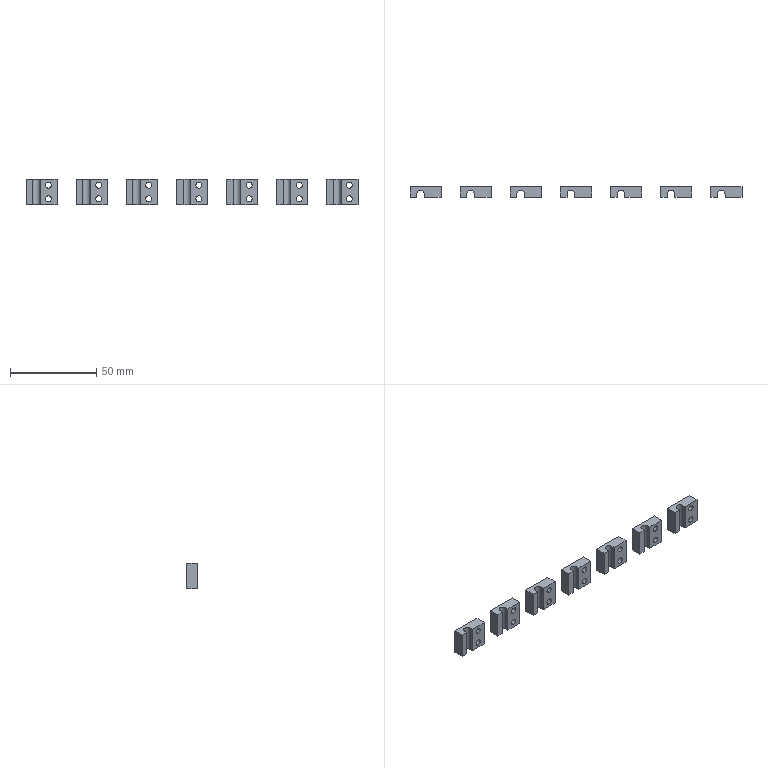Part | 7 solids | 98 faces | box 192 x 6 x 15 mm | volume 8902 mm3 | plane 63 | cylinder 35 | commonest cylinder face diameters 3.5 x28 4.4 x7